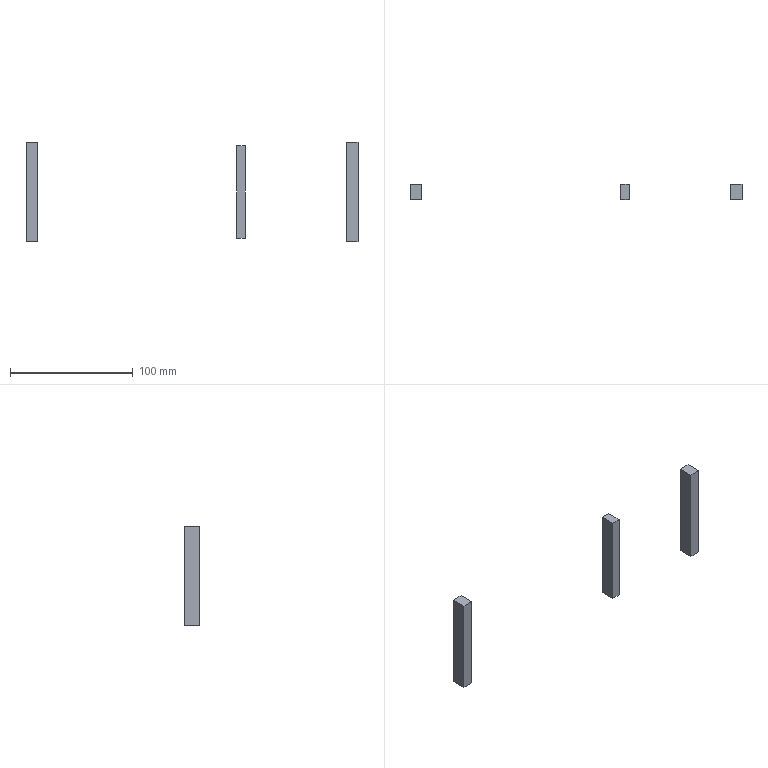Part | Mastercam | 3 solids | 18 faces | box 270.165 x 12.3 x 81 mm | volume 24955 mm3 | plane 18
STEP:
#1=CARTESIAN_POINT('',(0.,0.,0.));
#2=DIRECTION('',(0.,0.,1.));
#3=DIRECTION('',(1.,0.,0.));
#4=AXIS2_PLACEMENT_3D('',#1,#2,#3);
#5=CARTESIAN_POINT('',(-125.917,2.3,-40.5));
#6=VERTEX_POINT('',#5);
#7=CARTESIAN_POINT('',(-125.917,2.3,40.5));
#8=VERTEX_POINT('',#7);
#9=CARTESIAN_POINT('',(-125.917,2.3,-40.5));
#10=DIRECTION('',(0.,0.,1.));
#11=VECTOR('',#10,1.);
#12=LINE('',#9,#11);
#13=EDGE_CURVE('',#6,#8,#12,.T.);
#14=ORIENTED_EDGE('',*,*,#13,.T.);
#15=CARTESIAN_POINT('',(-125.917,-10.,40.5));
#16=VERTEX_POINT('',#15);
#17=CARTESIAN_POINT('',(-125.917,-10.,40.5));
#18=DIRECTION('',(0.,1.,0.));
#19=VECTOR('',#18,1.);
#20=LINE('',#17,#19);
#21=EDGE_CURVE('',#16,#8,#20,.T.);
#22=ORIENTED_EDGE('',*,*,#21,.F.);
#23=CARTESIAN_POINT('',(-125.917,-10.,-40.5));
#24=VERTEX_POINT('',#23);
#25=CARTESIAN_POINT('',(-125.917,-10.,-40.5));
#26=DIRECTION('',(0.,0.,1.));
#27=VECTOR('',#26,1.);
#28=LINE('',#25,#27);
#29=EDGE_CURVE('',#24,#16,#28,.T.);
#30=ORIENTED_EDGE('',*,*,#29,.F.);
#31=CARTESIAN_POINT('',(-125.917,-10.,-40.5));
#32=DIRECTION('',(0.,1.,0.));
#33=VECTOR('',#32,1.);
#34=LINE('',#31,#33);
#35=EDGE_CURVE('',#24,#6,#34,.T.);
#36=ORIENTED_EDGE('',*,*,#35,.T.);
#37=EDGE_LOOP('',(#14,#22,#30,#36));
#38=FACE_OUTER_BOUND('',#37,.T.);
#39=CARTESIAN_POINT('',(-125.917,-10.,-40.5));
#40=DIRECTION('',(-1.,0.,0.));
#41=DIRECTION('',(0.,0.,1.));
#42=AXIS2_PLACEMENT_3D('',#39,#40,#41);
#43=PLANE('',#42);
#44=ADVANCED_FACE('',(#38),#43,.F.);
#45=CARTESIAN_POINT('',(-135.083,2.3,40.5));
#46=VERTEX_POINT('',#45);
#47=CARTESIAN_POINT('',(-125.917,2.3,40.5));
#48=DIRECTION('',(-1.,0.,0.));
#49=VECTOR('',#48,1.);
#50=LINE('',#47,#49);
#51=EDGE_CURVE('',#8,#46,#50,.T.);
#52=ORIENTED_EDGE('',*,*,#51,.T.);
#53=CARTESIAN_POINT('',(-135.083,-10.,40.5));
#54=VERTEX_POINT('',#53);
#55=CARTESIAN_POINT('',(-135.083,-10.,40.5));
#56=DIRECTION('',(0.,1.,0.));
#57=VECTOR('',#56,1.);
#58=LINE('',#55,#57);
#59=EDGE_CURVE('',#54,#46,#58,.T.);
#60=ORIENTED_EDGE('',*,*,#59,.F.);
#61=CARTESIAN_POINT('',(-125.917,-10.,40.5));
#62=DIRECTION('',(-1.,0.,0.));
#63=VECTOR('',#62,1.);
#64=LINE('',#61,#63);
#65=EDGE_CURVE('',#16,#54,#64,.T.);
#66=ORIENTED_EDGE('',*,*,#65,.F.);
#67=ORIENTED_EDGE('',*,*,#21,.T.);
#68=EDGE_LOOP('',(#52,#60,#66,#67));
#69=FACE_OUTER_BOUND('',#68,.T.);
#70=CARTESIAN_POINT('',(-125.917,-10.,40.5));
#71=DIRECTION('',(0.,0.,-1.));
#72=DIRECTION('',(-1.,0.,0.));
#73=AXIS2_PLACEMENT_3D('',#70,#71,#72);
#74=PLANE('',#73);
#75=ADVANCED_FACE('',(#69),#74,.F.);
#76=CARTESIAN_POINT('',(-135.083,2.3,-40.5));
#77=VERTEX_POINT('',#76);
#78=CARTESIAN_POINT('',(-135.083,2.3,40.5));
#79=DIRECTION('',(0.,0.,-1.));
#80=VECTOR('',#79,1.);
#81=LINE('',#78,#80);
#82=EDGE_CURVE('',#46,#77,#81,.T.);
#83=ORIENTED_EDGE('',*,*,#82,.T.);
#84=CARTESIAN_POINT('',(-135.083,-10.,-40.5));
#85=VERTEX_POINT('',#84);
#86=CARTESIAN_POINT('',(-135.083,-10.,-40.5));
#87=DIRECTION('',(0.,1.,0.));
#88=VECTOR('',#87,1.);
#89=LINE('',#86,#88);
#90=EDGE_CURVE('',#85,#77,#89,.T.);
#91=ORIENTED_EDGE('',*,*,#90,.F.);
#92=CARTESIAN_POINT('',(-135.083,-10.,40.5));
#93=DIRECTION('',(0.,0.,-1.));
#94=VECTOR('',#93,1.);
#95=LINE('',#92,#94);
#96=EDGE_CURVE('',#54,#85,#95,.T.);
#97=ORIENTED_EDGE('',*,*,#96,.F.);
#98=ORIENTED_EDGE('',*,*,#59,.T.);
#99=EDGE_LOOP('',(#83,#91,#97,#98));
#100=FACE_OUTER_BOUND('',#99,.T.);
#101=CARTESIAN_POINT('',(-135.083,-10.,40.5));
#102=DIRECTION('',(1.,0.,0.));
#103=DIRECTION('',(0.,0.,-1.));
#104=AXIS2_PLACEMENT_3D('',#101,#102,#103);
#105=PLANE('',#104);
#106=ADVANCED_FACE('',(#100),#105,.F.);
#107=CARTESIAN_POINT('',(-135.083,2.3,-40.5));
#108=DIRECTION('',(1.,0.,0.));
#109=VECTOR('',#108,1.);
#110=LINE('',#107,#109);
#111=EDGE_CURVE('',#77,#6,#110,.T.);
#112=ORIENTED_EDGE('',*,*,#111,.T.);
#113=ORIENTED_EDGE('',*,*,#35,.F.);
#114=CARTESIAN_POINT('',(-135.083,-10.,-40.5));
#115=DIRECTION('',(1.,0.,0.));
#116=VECTOR('',#115,1.);
#117=LINE('',#114,#116);
#118=EDGE_CURVE('',#85,#24,#117,.T.);
#119=ORIENTED_EDGE('',*,*,#118,.F.);
#120=ORIENTED_EDGE('',*,*,#90,.T.);
#121=EDGE_LOOP('',(#112,#113,#119,#120));
#122=FACE_OUTER_BOUND('',#121,.T.);
#123=CARTESIAN_POINT('',(-135.083,-10.,-40.5));
#124=DIRECTION('',(0.,0.,1.));
#125=DIRECTION('',(1.,0.,0.));
#126=AXIS2_PLACEMENT_3D('',#123,#124,#125);
#127=PLANE('',#126);
#128=ADVANCED_FACE('',(#122),#127,.F.);
#129=ORIENTED_EDGE('',*,*,#29,.T.);
#130=ORIENTED_EDGE('',*,*,#65,.T.);
#131=ORIENTED_EDGE('',*,*,#96,.T.);
#132=ORIENTED_EDGE('',*,*,#118,.T.);
#133=EDGE_LOOP('',(#129,#130,#131,#132));
#134=FACE_OUTER_BOUND('',#133,.T.);
#135=CARTESIAN_POINT('',(0.,-10.,0.));
#136=DIRECTION('',(0.,-1.,0.));
#137=DIRECTION('',(0.,0.,-1.));
#138=AXIS2_PLACEMENT_3D('',#135,#136,#137);
#139=PLANE('',#138);
#140=ADVANCED_FACE('',(#134),#139,.T.);
#141=ORIENTED_EDGE('',*,*,#13,.F.);
#142=ORIENTED_EDGE('',*,*,#111,.F.);
#143=ORIENTED_EDGE('',*,*,#82,.F.);
#144=ORIENTED_EDGE('',*,*,#51,.F.);
#145=EDGE_LOOP('',(#141,#142,#143,#144));
#146=FACE_OUTER_BOUND('',#145,.T.);
#147=CARTESIAN_POINT('',(0.,2.3,0.));
#148=DIRECTION('',(0.,-1.,0.));
#149=DIRECTION('',(0.,0.,-1.));
#150=AXIS2_PLACEMENT_3D('',#147,#148,#149);
#151=PLANE('',#150);
#152=ADVANCED_FACE('',(#146),#151,.F.);
#153=CLOSED_SHELL('',(#44,#75,#106,#128,#140,#152));
#154=MANIFOLD_SOLID_BREP('',#153);
#155=CARTESIAN_POINT('',(43.5,2.3,-37.5));
#156=VERTEX_POINT('',#155);
#157=CARTESIAN_POINT('',(43.5,2.3,37.5));
#158=VERTEX_POINT('',#157);
#159=CARTESIAN_POINT('',(43.5,2.3,-37.5));
#160=DIRECTION('',(0.,0.,1.));
#161=VECTOR('',#160,1.);
#162=LINE('',#159,#161);
#163=EDGE_CURVE('',#156,#158,#162,.T.);
#164=ORIENTED_EDGE('',*,*,#163,.T.);
#165=CARTESIAN_POINT('',(43.5,-10.,37.5));
#166=VERTEX_POINT('',#165);
#167=CARTESIAN_POINT('',(43.5,-10.,37.5));
#168=DIRECTION('',(0.,1.,0.));
#169=VECTOR('',#168,1.);
#170=LINE('',#167,#169);
#171=EDGE_CURVE('',#166,#158,#170,.T.);
#172=ORIENTED_EDGE('',*,*,#171,.F.);
#173=CARTESIAN_POINT('',(43.5,-10.,-37.5));
#174=VERTEX_POINT('',#173);
#175=CARTESIAN_POINT('',(43.5,-10.,-37.5));
#176=DIRECTION('',(0.,0.,1.));
#177=VECTOR('',#176,1.);
#178=LINE('',#175,#177);
#179=EDGE_CURVE('',#174,#166,#178,.T.);
#180=ORIENTED_EDGE('',*,*,#179,.F.);
#181=CARTESIAN_POINT('',(43.5,-10.,-37.5));
#182=DIRECTION('',(0.,1.,0.));
#183=VECTOR('',#182,1.);
#184=LINE('',#181,#183);
#185=EDGE_CURVE('',#174,#156,#184,.T.);
#186=ORIENTED_EDGE('',*,*,#185,.T.);
#187=EDGE_LOOP('',(#164,#172,#180,#186));
#188=FACE_OUTER_BOUND('',#187,.T.);
#189=CARTESIAN_POINT('',(43.5,-10.,-37.5));
#190=DIRECTION('',(-1.,0.,0.));
#191=DIRECTION('',(0.,0.,1.));
#192=AXIS2_PLACEMENT_3D('',#189,#190,#191);
#193=PLANE('',#192);
#194=ADVANCED_FACE('',(#188),#193,.F.);
#195=CARTESIAN_POINT('',(36.245,2.3,37.5));
#196=VERTEX_POINT('',#195);
#197=CARTESIAN_POINT('',(43.5,2.3,37.5));
#198=DIRECTION('',(-1.,0.,0.));
#199=VECTOR('',#198,1.);
#200=LINE('',#197,#199);
#201=EDGE_CURVE('',#158,#196,#200,.T.);
#202=ORIENTED_EDGE('',*,*,#201,.T.);
#203=CARTESIAN_POINT('',(36.245,-10.,37.5));
#204=VERTEX_POINT('',#203);
#205=CARTESIAN_POINT('',(36.245,-10.,37.5));
#206=DIRECTION('',(0.,1.,0.));
#207=VECTOR('',#206,1.);
#208=LINE('',#205,#207);
#209=EDGE_CURVE('',#204,#196,#208,.T.);
#210=ORIENTED_EDGE('',*,*,#209,.F.);
#211=CARTESIAN_POINT('',(43.5,-10.,37.5));
#212=DIRECTION('',(-1.,0.,0.));
#213=VECTOR('',#212,1.);
#214=LINE('',#211,#213);
#215=EDGE_CURVE('',#166,#204,#214,.T.);
#216=ORIENTED_EDGE('',*,*,#215,.F.);
#217=ORIENTED_EDGE('',*,*,#171,.T.);
#218=EDGE_LOOP('',(#202,#210,#216,#217));
#219=FACE_OUTER_BOUND('',#218,.T.);
#220=CARTESIAN_POINT('',(43.5,-10.,37.5));
#221=DIRECTION('',(0.,0.,-1.));
#222=DIRECTION('',(-1.,0.,0.));
#223=AXIS2_PLACEMENT_3D('',#220,#221,#222);
#224=PLANE('',#223);
#225=ADVANCED_FACE('',(#219),#224,.F.);
#226=CARTESIAN_POINT('',(36.245,2.3,-37.5));
#227=VERTEX_POINT('',#226);
#228=CARTESIAN_POINT('',(36.245,2.3,37.5));
#229=DIRECTION('',(0.,0.,-1.));
#230=VECTOR('',#229,1.);
#231=LINE('',#228,#230);
#232=EDGE_CURVE('',#196,#227,#231,.T.);
#233=ORIENTED_EDGE('',*,*,#232,.T.);
#234=CARTESIAN_POINT('',(36.245,-10.,-37.5));
#235=VERTEX_POINT('',#234);
#236=CARTESIAN_POINT('',(36.245,-10.,-37.5));
#237=DIRECTION('',(0.,1.,0.));
#238=VECTOR('',#237,1.);
#239=LINE('',#236,#238);
#240=EDGE_CURVE('',#235,#227,#239,.T.);
#241=ORIENTED_EDGE('',*,*,#240,.F.);
#242=CARTESIAN_POINT('',(36.245,-10.,37.5));
#243=DIRECTION('',(0.,0.,-1.));
#244=VECTOR('',#243,1.);
#245=LINE('',#242,#244);
#246=EDGE_CURVE('',#204,#235,#245,.T.);
#247=ORIENTED_EDGE('',*,*,#246,.F.);
#248=ORIENTED_EDGE('',*,*,#209,.T.);
#249=EDGE_LOOP('',(#233,#241,#247,#248));
#250=FACE_OUTER_BOUND('',#249,.T.);
#251=CARTESIAN_POINT('',(36.245,-10.,37.5));
#252=DIRECTION('',(1.,0.,0.));
#253=DIRECTION('',(0.,0.,-1.));
#254=AXIS2_PLACEMENT_3D('',#251,#252,#253);
#255=PLANE('',#254);
#256=ADVANCED_FACE('',(#250),#255,.F.);
#257=CARTESIAN_POINT('',(36.245,2.3,-37.5));
#258=DIRECTION('',(1.,0.,0.));
#259=VECTOR('',#258,1.);
#260=LINE('',#257,#259);
#261=EDGE_CURVE('',#227,#156,#260,.T.);
#262=ORIENTED_EDGE('',*,*,#261,.T.);
#263=ORIENTED_EDGE('',*,*,#185,.F.);
#264=CARTESIAN_POINT('',(36.245,-10.,-37.5));
#265=DIRECTION('',(1.,0.,0.));
#266=VECTOR('',#265,1.);
#267=LINE('',#264,#266);
#268=EDGE_CURVE('',#235,#174,#267,.T.);
#269=ORIENTED_EDGE('',*,*,#268,.F.);
#270=ORIENTED_EDGE('',*,*,#240,.T.);
#271=EDGE_LOOP('',(#262,#263,#269,#270));
#272=FACE_OUTER_BOUND('',#271,.T.);
#273=CARTESIAN_POINT('',(36.245,-10.,-37.5));
#274=DIRECTION('',(0.,0.,1.));
#275=DIRECTION('',(1.,0.,0.));
#276=AXIS2_PLACEMENT_3D('',#273,#274,#275);
#277=PLANE('',#276);
#278=ADVANCED_FACE('',(#272),#277,.F.);
#279=ORIENTED_EDGE('',*,*,#179,.T.);
#280=ORIENTED_EDGE('',*,*,#215,.T.);
#281=ORIENTED_EDGE('',*,*,#246,.T.);
#282=ORIENTED_EDGE('',*,*,#268,.T.);
#283=EDGE_LOOP('',(#279,#280,#281,#282));
#284=FACE_OUTER_BOUND('',#283,.T.);
#285=CARTESIAN_POINT('',(0.,-10.,0.));
#286=DIRECTION('',(0.,-1.,0.));
#287=DIRECTION('',(0.,0.,-1.));
#288=AXIS2_PLACEMENT_3D('',#285,#286,#287);
#289=PLANE('',#288);
#290=ADVANCED_FACE('',(#284),#289,.T.);
#291=ORIENTED_EDGE('',*,*,#163,.F.);
#292=ORIENTED_EDGE('',*,*,#261,.F.);
#293=ORIENTED_EDGE('',*,*,#232,.F.);
#294=ORIENTED_EDGE('',*,*,#201,.F.);
#295=EDGE_LOOP('',(#291,#292,#293,#294));
#296=FACE_OUTER_BOUND('',#295,.T.);
#297=CARTESIAN_POINT('',(0.,2.3,0.));
#298=DIRECTION('',(0.,-1.,0.));
#299=DIRECTION('',(0.,0.,-1.));
#300=AXIS2_PLACEMENT_3D('',#297,#298,#299);
#301=PLANE('',#300);
#302=ADVANCED_FACE('',(#296),#301,.F.);
#303=CLOSED_SHELL('',(#194,#225,#256,#278,#290,#302));
#304=MANIFOLD_SOLID_BREP('',#303);
#305=CARTESIAN_POINT('',(135.083,2.3,-40.5));
#306=VERTEX_POINT('',#305);
#307=CARTESIAN_POINT('',(135.083,2.3,40.5));
#308=VERTEX_POINT('',#307);
#309=CARTESIAN_POINT('',(135.083,2.3,-40.5));
#310=DIRECTION('',(0.,0.,1.));
#311=VECTOR('',#310,1.);
#312=LINE('',#309,#311);
#313=EDGE_CURVE('',#306,#308,#312,.T.);
#314=ORIENTED_EDGE('',*,*,#313,.T.);
#315=CARTESIAN_POINT('',(135.083,-10.,40.5));
#316=VERTEX_POINT('',#315);
#317=CARTESIAN_POINT('',(135.083,-10.,40.5));
#318=DIRECTION('',(0.,1.,0.));
#319=VECTOR('',#318,1.);
#320=LINE('',#317,#319);
#321=EDGE_CURVE('',#316,#308,#320,.T.);
#322=ORIENTED_EDGE('',*,*,#321,.F.);
#323=CARTESIAN_POINT('',(135.083,-10.,-40.5));
#324=VERTEX_POINT('',#323);
#325=CARTESIAN_POINT('',(135.083,-10.,-40.5));
#326=DIRECTION('',(0.,0.,1.));
#327=VECTOR('',#326,1.);
#328=LINE('',#325,#327);
#329=EDGE_CURVE('',#324,#316,#328,.T.);
#330=ORIENTED_EDGE('',*,*,#329,.F.);
#331=CARTESIAN_POINT('',(135.083,-10.,-40.5));
#332=DIRECTION('',(0.,1.,0.));
#333=VECTOR('',#332,1.);
#334=LINE('',#331,#333);
#335=EDGE_CURVE('',#324,#306,#334,.T.);
#336=ORIENTED_EDGE('',*,*,#335,.T.);
#337=EDGE_LOOP('',(#314,#322,#330,#336));
#338=FACE_OUTER_BOUND('',#337,.T.);
#339=CARTESIAN_POINT('',(135.083,-10.,-40.5));
#340=DIRECTION('',(-1.,0.,0.));
#341=DIRECTION('',(0.,0.,1.));
#342=AXIS2_PLACEMENT_3D('',#339,#340,#341);
#343=PLANE('',#342);
#344=ADVANCED_FACE('',(#338),#343,.F.);
#345=CARTESIAN_POINT('',(125.917,2.3,40.5));
#346=VERTEX_POINT('',#345);
#347=CARTESIAN_POINT('',(135.083,2.3,40.5));
#348=DIRECTION('',(-1.,0.,0.));
#349=VECTOR('',#348,1.);
#350=LINE('',#347,#349);
#351=EDGE_CURVE('',#308,#346,#350,.T.);
#352=ORIENTED_EDGE('',*,*,#351,.T.);
#353=CARTESIAN_POINT('',(125.917,-10.,40.5));
#354=VERTEX_POINT('',#353);
#355=CARTESIAN_POINT('',(125.917,-10.,40.5));
#356=DIRECTION('',(0.,1.,0.));
#357=VECTOR('',#356,1.);
#358=LINE('',#355,#357);
#359=EDGE_CURVE('',#354,#346,#358,.T.);
#360=ORIENTED_EDGE('',*,*,#359,.F.);
#361=CARTESIAN_POINT('',(135.083,-10.,40.5));
#362=DIRECTION('',(-1.,0.,0.));
#363=VECTOR('',#362,1.);
#364=LINE('',#361,#363);
#365=EDGE_CURVE('',#316,#354,#364,.T.);
#366=ORIENTED_EDGE('',*,*,#365,.F.);
#367=ORIENTED_EDGE('',*,*,#321,.T.);
#368=EDGE_LOOP('',(#352,#360,#366,#367));
#369=FACE_OUTER_BOUND('',#368,.T.);
#370=CARTESIAN_POINT('',(135.083,-10.,40.5));
#371=DIRECTION('',(0.,0.,-1.));
#372=DIRECTION('',(-1.,0.,0.));
#373=AXIS2_PLACEMENT_3D('',#370,#371,#372);
#374=PLANE('',#373);
#375=ADVANCED_FACE('',(#369),#374,.F.);
#376=CARTESIAN_POINT('',(125.917,2.3,-40.5));
#377=VERTEX_POINT('',#376);
#378=CARTESIAN_POINT('',(125.917,2.3,40.5));
#379=DIRECTION('',(0.,0.,-1.));
#380=VECTOR('',#379,1.);
#381=LINE('',#378,#380);
#382=EDGE_CURVE('',#346,#377,#381,.T.);
#383=ORIENTED_EDGE('',*,*,#382,.T.);
#384=CARTESIAN_POINT('',(125.917,-10.,-40.5));
#385=VERTEX_POINT('',#384);
#386=CARTESIAN_POINT('',(125.917,-10.,-40.5));
#387=DIRECTION('',(0.,1.,0.));
#388=VECTOR('',#387,1.);
#389=LINE('',#386,#388);
#390=EDGE_CURVE('',#385,#377,#389,.T.);
#391=ORIENTED_EDGE('',*,*,#390,.F.);
#392=CARTESIAN_POINT('',(125.917,-10.,40.5));
#393=DIRECTION('',(0.,0.,-1.));
#394=VECTOR('',#393,1.);
#395=LINE('',#392,#394);
#396=EDGE_CURVE('',#354,#385,#395,.T.);
#397=ORIENTED_EDGE('',*,*,#396,.F.);
#398=ORIENTED_EDGE('',*,*,#359,.T.);
#399=EDGE_LOOP('',(#383,#391,#397,#398));
#400=FACE_OUTER_BOUND('',#399,.T.);
#401=CARTESIAN_POINT('',(125.917,-10.,40.5));
#402=DIRECTION('',(1.,0.,0.));
#403=DIRECTION('',(0.,0.,-1.));
#404=AXIS2_PLACEMENT_3D('',#401,#402,#403);
#405=PLANE('',#404);
#406=ADVANCED_FACE('',(#400),#405,.F.);
#407=CARTESIAN_POINT('',(125.917,2.3,-40.5));
#408=DIRECTION('',(1.,0.,0.));
#409=VECTOR('',#408,1.);
#410=LINE('',#407,#409);
#411=EDGE_CURVE('',#377,#306,#410,.T.);
#412=ORIENTED_EDGE('',*,*,#411,.T.);
#413=ORIENTED_EDGE('',*,*,#335,.F.);
#414=CARTESIAN_POINT('',(125.917,-10.,-40.5));
#415=DIRECTION('',(1.,0.,0.));
#416=VECTOR('',#415,1.);
#417=LINE('',#414,#416);
#418=EDGE_CURVE('',#385,#324,#417,.T.);
#419=ORIENTED_EDGE('',*,*,#418,.F.);
#420=ORIENTED_EDGE('',*,*,#390,.T.);
#421=EDGE_LOOP('',(#412,#413,#419,#420));
#422=FACE_OUTER_BOUND('',#421,.T.);
#423=CARTESIAN_POINT('',(125.917,-10.,-40.5));
#424=DIRECTION('',(0.,0.,1.));
#425=DIRECTION('',(1.,0.,0.));
#426=AXIS2_PLACEMENT_3D('',#423,#424,#425);
#427=PLANE('',#426);
#428=ADVANCED_FACE('',(#422),#427,.F.);
#429=ORIENTED_EDGE('',*,*,#329,.T.);
#430=ORIENTED_EDGE('',*,*,#365,.T.);
#431=ORIENTED_EDGE('',*,*,#396,.T.);
#432=ORIENTED_EDGE('',*,*,#418,.T.);
#433=EDGE_LOOP('',(#429,#430,#431,#432));
#434=FACE_OUTER_BOUND('',#433,.T.);
#435=CARTESIAN_POINT('',(0.,-10.,0.));
#436=DIRECTION('',(0.,-1.,0.));
#437=DIRECTION('',(0.,0.,-1.));
#438=AXIS2_PLACEMENT_3D('',#435,#436,#437);
#439=PLANE('',#438);
#440=ADVANCED_FACE('',(#434),#439,.T.);
#441=ORIENTED_EDGE('',*,*,#313,.F.);
#442=ORIENTED_EDGE('',*,*,#411,.F.);
#443=ORIENTED_EDGE('',*,*,#382,.F.);
#444=ORIENTED_EDGE('',*,*,#351,.F.);
#445=EDGE_LOOP('',(#441,#442,#443,#444));
#446=FACE_OUTER_BOUND('',#445,.T.);
#447=CARTESIAN_POINT('',(0.,2.3,0.));
#448=DIRECTION('',(0.,-1.,0.));
#449=DIRECTION('',(0.,0.,-1.));
#450=AXIS2_PLACEMENT_3D('',#447,#448,#449);
#451=PLANE('',#450);
#452=ADVANCED_FACE('',(#446),#451,.F.);
#453=CLOSED_SHELL('',(#344,#375,#406,#428,#440,#452));
#454=MANIFOLD_SOLID_BREP('',#453);
#455=(LENGTH_UNIT()NAMED_UNIT(*)SI_UNIT(.MILLI.,.METRE.));
#456=UNCERTAINTY_MEASURE_WITH_UNIT(LENGTH_MEASURE(0.005),#455,'','');
#457=(NAMED_UNIT(*)PLANE_ANGLE_UNIT()SI_UNIT($,.RADIAN.));
#458=(GEOMETRIC_REPRESENTATION_CONTEXT(3)GLOBAL_UNCERTAINTY_ASSIGNED_CONTEXT((#456))GLOBAL_UNIT_ASSIGNED_CONTEXT((#455,#457))REPRESENTATION_CONTEXT('',''));
#459=ADVANCED_BREP_SHAPE_REPRESENTATION('',(#4,#154,#304,#454),#458);